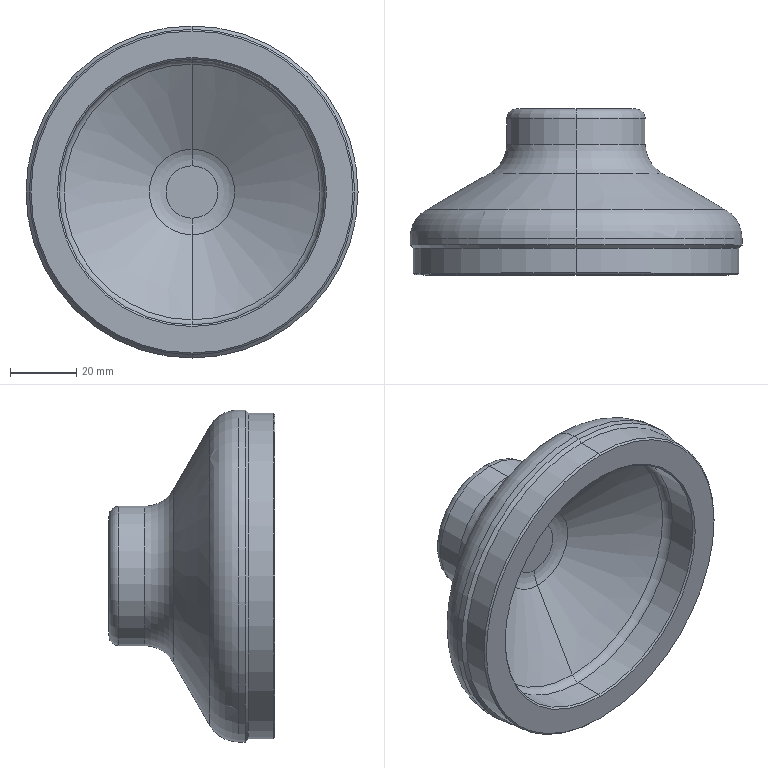Part | NX | features BREP 1 | 1 solid | 38 faces | box 100 x 50 x 100 mm | volume 123774 mm3 | cone 12 | cylinder 10 | torus 10 | plane 4 | sphere 2 | commonest cylinder face diameters 28 x2 42 x2 80 x2 98 x2 100 x2
STEP:
#1=CARTESIAN_POINT('',(0.,-49.5,40.));
#2=VERTEX_POINT('',#1);
#3=CARTESIAN_POINT('',(0.,-49.5,-40.));
#4=VERTEX_POINT('',#3);
#5=CARTESIAN_POINT('',(0.,-49.5,0.));
#6=DIRECTION('',(0.,-1.,0.));
#7=DIRECTION('',(0.,0.,1.));
#8=AXIS2_PLACEMENT_3D('',#5,#6,#7);
#9=CIRCLE('',#8,40.);
#10=EDGE_CURVE('',#2,#4,#9,.T.);
#11=ORIENTED_EDGE('',*,*,#10,.F.);
#12=CARTESIAN_POINT('',(0.,-50.,40.5));
#13=VERTEX_POINT('',#12);
#14=CARTESIAN_POINT('',(0.,-50.,40.5));
#15=DIRECTION('',(0.,-0.7071,0.7071));
#16=VECTOR('',#15,1000.);
#17=LINE('',#14,#16);
#18=EDGE_CURVE('',#2,#13,#17,.T.);
#19=ORIENTED_EDGE('',*,*,#18,.T.);
#20=CARTESIAN_POINT('',(0.,-50.,-40.5));
#21=VERTEX_POINT('',#20);
#22=CARTESIAN_POINT('',(0.,-50.,0.));
#23=DIRECTION('',(0.,1.,0.));
#24=DIRECTION('',(0.,0.,1.));
#25=AXIS2_PLACEMENT_3D('',#22,#23,#24);
#26=CIRCLE('',#25,40.5);
#27=EDGE_CURVE('',#21,#13,#26,.T.);
#28=ORIENTED_EDGE('',*,*,#27,.F.);
#29=CARTESIAN_POINT('',(0.,-50.,-40.5));
#30=DIRECTION('',(0.,-0.7071,-0.7071));
#31=VECTOR('',#30,1000.);
#32=LINE('',#29,#31);
#33=EDGE_CURVE('',#4,#21,#32,.T.);
#34=ORIENTED_EDGE('',*,*,#33,.F.);
#35=EDGE_LOOP('',(#11,#19,#28,#34));
#36=FACE_BOUND('',#35,.T.);
#37=CARTESIAN_POINT('',(0.,-50.,0.));
#38=DIRECTION('',(0.,-1.,0.));
#39=DIRECTION('',(0.,0.,-1.));
#40=AXIS2_PLACEMENT_3D('',#37,#38,#39);
#41=CONICAL_SURFACE('',#40,40.5,0.7854);
#42=ADVANCED_FACE('',(#36),#41,.F.);
#43=CARTESIAN_POINT('',(0.,-50.,-48.5));
#44=VERTEX_POINT('',#43);
#45=CARTESIAN_POINT('',(0.,-50.,48.5));
#46=VERTEX_POINT('',#45);
#47=CARTESIAN_POINT('',(0.,-50.,0.));
#48=DIRECTION('',(0.,-1.,0.));
#49=DIRECTION('',(0.,0.,1.));
#50=AXIS2_PLACEMENT_3D('',#47,#48,#49);
#51=CIRCLE('',#50,48.5);
#52=EDGE_CURVE('',#44,#46,#51,.T.);
#53=ORIENTED_EDGE('',*,*,#52,.F.);
#54=CARTESIAN_POINT('',(0.,-49.5,-49.));
#55=VERTEX_POINT('',#54);
#56=CARTESIAN_POINT('',(0.,-50.,-48.5));
#57=DIRECTION('',(0.,0.7071,-0.7071));
#58=VECTOR('',#57,1000.);
#59=LINE('',#56,#58);
#60=EDGE_CURVE('',#55,#44,#59,.F.);
#61=ORIENTED_EDGE('',*,*,#60,.F.);
#62=CARTESIAN_POINT('',(0.,-49.5,49.));
#63=VERTEX_POINT('',#62);
#64=CARTESIAN_POINT('',(0.,-49.5,0.));
#65=DIRECTION('',(0.,1.,0.));
#66=DIRECTION('',(0.,0.,1.));
#67=AXIS2_PLACEMENT_3D('',#64,#65,#66);
#68=CIRCLE('',#67,49.);
#69=EDGE_CURVE('',#63,#55,#68,.T.);
#70=ORIENTED_EDGE('',*,*,#69,.F.);
#71=CARTESIAN_POINT('',(0.,-50.,48.5));
#72=DIRECTION('',(0.,0.7071,0.7071));
#73=VECTOR('',#72,1000.);
#74=LINE('',#71,#73);
#75=EDGE_CURVE('',#63,#46,#74,.F.);
#76=ORIENTED_EDGE('',*,*,#75,.T.);
#77=EDGE_LOOP('',(#53,#61,#70,#76));
#78=FACE_BOUND('',#77,.T.);
#79=CARTESIAN_POINT('',(0.,-50.,0.));
#80=DIRECTION('',(0.,1.,0.));
#81=DIRECTION('',(0.,0.,1.));
#82=AXIS2_PLACEMENT_3D('',#79,#80,#81);
#83=CONICAL_SURFACE('',#82,48.5,0.7854);
#84=ADVANCED_FACE('',(#78),#83,.T.);
#85=CARTESIAN_POINT('',(0.,-42.,-49.));
#86=VERTEX_POINT('',#85);
#87=CARTESIAN_POINT('',(0.,-42.,49.));
#88=VERTEX_POINT('',#87);
#89=CARTESIAN_POINT('',(0.,-42.,0.));
#90=DIRECTION('',(0.,-1.,0.));
#91=DIRECTION('',(0.,0.,-1.));
#92=AXIS2_PLACEMENT_3D('',#89,#90,#91);
#93=CIRCLE('',#92,49.);
#94=EDGE_CURVE('',#86,#88,#93,.T.);
#95=ORIENTED_EDGE('',*,*,#94,.F.);
#96=CARTESIAN_POINT('',(0.,-41.,-50.));
#97=VERTEX_POINT('',#96);
#98=CARTESIAN_POINT('',(0.,-42.,-49.));
#99=DIRECTION('',(0.,0.7071,-0.7071));
#100=VECTOR('',#99,1000.);
#101=LINE('',#98,#100);
#102=EDGE_CURVE('',#97,#86,#101,.F.);
#103=ORIENTED_EDGE('',*,*,#102,.F.);
#104=CARTESIAN_POINT('',(0.,-41.,50.));
#105=VERTEX_POINT('',#104);
#106=CARTESIAN_POINT('',(0.,-41.,0.));
#107=DIRECTION('',(0.,1.,0.));
#108=DIRECTION('',(0.,0.,-1.));
#109=AXIS2_PLACEMENT_3D('',#106,#107,#108);
#110=CIRCLE('',#109,50.);
#111=EDGE_CURVE('',#105,#97,#110,.T.);
#112=ORIENTED_EDGE('',*,*,#111,.F.);
#113=CARTESIAN_POINT('',(0.,-42.,49.));
#114=DIRECTION('',(0.,0.7071,0.7071));
#115=VECTOR('',#114,1000.);
#116=LINE('',#113,#115);
#117=EDGE_CURVE('',#105,#88,#116,.F.);
#118=ORIENTED_EDGE('',*,*,#117,.T.);
#119=EDGE_LOOP('',(#95,#103,#112,#118));
#120=FACE_BOUND('',#119,.T.);
#121=CARTESIAN_POINT('',(0.,-42.,0.));
#122=DIRECTION('',(0.,1.,0.));
#123=DIRECTION('',(0.,0.,1.));
#124=AXIS2_PLACEMENT_3D('',#121,#122,#123);
#125=CONICAL_SURFACE('',#124,49.,0.7854);
#126=ADVANCED_FACE('',(#120),#125,.T.);
#127=ORIENTED_EDGE('',*,*,#10,.T.);
#128=CARTESIAN_POINT('',(0.,-40.732,-40.));
#129=VERTEX_POINT('',#128);
#130=CARTESIAN_POINT('',(0.,0.,-40.));
#131=DIRECTION('',(0.,1.,0.));
#132=VECTOR('',#131,1000.);
#133=LINE('',#130,#132);
#134=EDGE_CURVE('',#129,#4,#133,.F.);
#135=ORIENTED_EDGE('',*,*,#134,.F.);
#136=CARTESIAN_POINT('',(0.,-40.732,40.));
#137=VERTEX_POINT('',#136);
#138=CARTESIAN_POINT('',(0.,-40.732,0.));
#139=DIRECTION('',(0.,1.,0.));
#140=DIRECTION('',(0.,0.,1.));
#141=AXIS2_PLACEMENT_3D('',#138,#139,#140);
#142=CIRCLE('',#141,40.);
#143=EDGE_CURVE('',#129,#137,#142,.T.);
#144=ORIENTED_EDGE('',*,*,#143,.T.);
#145=CARTESIAN_POINT('',(0.,0.,40.));
#146=DIRECTION('',(0.,1.,0.));
#147=VECTOR('',#146,1000.);
#148=LINE('',#145,#147);
#149=EDGE_CURVE('',#137,#2,#148,.F.);
#150=ORIENTED_EDGE('',*,*,#149,.T.);
#151=EDGE_LOOP('',(#127,#135,#144,#150));
#152=FACE_BOUND('',#151,.T.);
#153=CARTESIAN_POINT('',(0.,0.,0.));
#154=DIRECTION('',(0.,1.,0.));
#155=DIRECTION('',(0.,0.,1.));
#156=AXIS2_PLACEMENT_3D('',#153,#154,#155);
#157=CYLINDRICAL_SURFACE('',#156,40.);
#158=ADVANCED_FACE('',(#152),#157,.F.);
#159=ORIENTED_EDGE('',*,*,#143,.F.);
#160=CARTESIAN_POINT('',(0.,-38.134,-38.5));
#161=VERTEX_POINT('',#160);
#162=CARTESIAN_POINT('',(0.,-40.732,-37.));
#163=DIRECTION('',(1.,0.,0.));
#164=DIRECTION('',(0.,0.,-1.));
#165=AXIS2_PLACEMENT_3D('',#162,#163,#164);
#166=CIRCLE('',#165,3.);
#167=EDGE_CURVE('',#161,#129,#166,.F.);
#168=ORIENTED_EDGE('',*,*,#167,.F.);
#169=CARTESIAN_POINT('',(0.,-38.134,38.5));
#170=VERTEX_POINT('',#169);
#171=CARTESIAN_POINT('',(0.,-38.134,0.));
#172=DIRECTION('',(0.,-1.,0.));
#173=DIRECTION('',(0.,0.,-1.));
#174=AXIS2_PLACEMENT_3D('',#171,#172,#173);
#175=CIRCLE('',#174,38.5);
#176=EDGE_CURVE('',#170,#161,#175,.T.);
#177=ORIENTED_EDGE('',*,*,#176,.F.);
#178=CARTESIAN_POINT('',(0.,-40.732,37.));
#179=DIRECTION('',(-1.,0.,0.));
#180=DIRECTION('',(0.,0.,1.));
#181=AXIS2_PLACEMENT_3D('',#178,#179,#180);
#182=CIRCLE('',#181,3.);
#183=EDGE_CURVE('',#170,#137,#182,.F.);
#184=ORIENTED_EDGE('',*,*,#183,.T.);
#185=EDGE_LOOP('',(#159,#168,#177,#184));
#186=FACE_BOUND('',#185,.T.);
#187=CARTESIAN_POINT('',(0.,-40.732,0.));
#188=DIRECTION('',(0.,1.,0.));
#189=DIRECTION('',(0.,0.,1.));
#190=AXIS2_PLACEMENT_3D('',#187,#188,#189);
#191=TOROIDAL_SURFACE('',#190,37.,3.);
#192=ADVANCED_FACE('',(#186),#191,.F.);
#193=CARTESIAN_POINT('',(0.,-23.34,-12.876));
#194=VERTEX_POINT('',#193);
#195=CARTESIAN_POINT('',(0.,-23.34,12.876));
#196=VERTEX_POINT('',#195);
#197=CARTESIAN_POINT('',(0.,-23.34,0.));
#198=DIRECTION('',(0.,1.,0.));
#199=DIRECTION('',(0.,0.,-1.));
#200=AXIS2_PLACEMENT_3D('',#197,#198,#199);
#201=CIRCLE('',#200,12.876);
#202=EDGE_CURVE('',#194,#196,#201,.T.);
#203=ORIENTED_EDGE('',*,*,#202,.T.);
#204=CARTESIAN_POINT('',(0.,-22.,10.555));
#205=DIRECTION('',(0.,-0.5,0.866));
#206=VECTOR('',#205,1000.);
#207=LINE('',#204,#206);
#208=EDGE_CURVE('',#196,#170,#207,.T.);
#209=ORIENTED_EDGE('',*,*,#208,.T.);
#210=ORIENTED_EDGE('',*,*,#176,.T.);
#211=CARTESIAN_POINT('',(0.,-22.,-10.555));
#212=DIRECTION('',(0.,-0.5,-0.866));
#213=VECTOR('',#212,1000.);
#214=LINE('',#211,#213);
#215=EDGE_CURVE('',#194,#161,#214,.T.);
#216=ORIENTED_EDGE('',*,*,#215,.F.);
#217=EDGE_LOOP('',(#203,#209,#210,#216));
#218=FACE_BOUND('',#217,.T.);
#219=CARTESIAN_POINT('',(0.,-22.,0.));
#220=DIRECTION('',(0.,-1.,0.));
#221=DIRECTION('',(0.,0.,-1.));
#222=AXIS2_PLACEMENT_3D('',#219,#220,#221);
#223=CONICAL_SURFACE('',#222,10.555,1.047);
#224=ADVANCED_FACE('',(#218),#223,.F.);
#225=ORIENTED_EDGE('',*,*,#202,.F.);
#226=CARTESIAN_POINT('',(0.,-22.,-7.876));
#227=VERTEX_POINT('',#226);
#228=CARTESIAN_POINT('',(0.,-32.,-7.876));
#229=DIRECTION('',(1.,0.,0.));
#230=DIRECTION('',(0.,0.,-1.));
#231=AXIS2_PLACEMENT_3D('',#228,#229,#230);
#232=CIRCLE('',#231,10.);
#233=EDGE_CURVE('',#227,#194,#232,.F.);
#234=ORIENTED_EDGE('',*,*,#233,.F.);
#235=CARTESIAN_POINT('',(0.,-22.,7.876));
#236=VERTEX_POINT('',#235);
#237=CARTESIAN_POINT('',(0.,-22.,0.));
#238=DIRECTION('',(0.,-1.,0.));
#239=DIRECTION('',(0.,0.,1.));
#240=AXIS2_PLACEMENT_3D('',#237,#238,#239);
#241=CIRCLE('',#240,7.876);
#242=EDGE_CURVE('',#236,#227,#241,.T.);
#243=ORIENTED_EDGE('',*,*,#242,.F.);
#244=CARTESIAN_POINT('',(0.,-32.,7.876));
#245=DIRECTION('',(-1.,0.,0.));
#246=DIRECTION('',(0.,0.,1.));
#247=AXIS2_PLACEMENT_3D('',#244,#245,#246);
#248=CIRCLE('',#247,10.);
#249=EDGE_CURVE('',#236,#196,#248,.F.);
#250=ORIENTED_EDGE('',*,*,#249,.T.);
#251=EDGE_LOOP('',(#225,#234,#243,#250));
#252=FACE_BOUND('',#251,.T.);
#253=CARTESIAN_POINT('',(0.,-32.,0.));
#254=DIRECTION('',(0.,1.,0.));
#255=DIRECTION('',(0.,0.,1.));
#256=AXIS2_PLACEMENT_3D('',#253,#254,#255);
#257=DEGENERATE_TOROIDAL_SURFACE('',#256,7.876,10.,.T.);
#258=ADVANCED_FACE('',(#252),#257,.F.);
#259=ORIENTED_EDGE('',*,*,#94,.T.);
#260=CARTESIAN_POINT('',(0.,-42.,49.));
#261=DIRECTION('',(0.,-1.,0.));
#262=VECTOR('',#261,1000.);
#263=LINE('',#260,#262);
#264=EDGE_CURVE('',#88,#63,#263,.T.);
#265=ORIENTED_EDGE('',*,*,#264,.T.);
#266=ORIENTED_EDGE('',*,*,#69,.T.);
#267=CARTESIAN_POINT('',(0.,-42.,-49.));
#268=DIRECTION('',(0.,-1.,0.));
#269=VECTOR('',#268,1000.);
#270=LINE('',#267,#269);
#271=EDGE_CURVE('',#86,#55,#270,.T.);
#272=ORIENTED_EDGE('',*,*,#271,.F.);
#273=EDGE_LOOP('',(#259,#265,#266,#272));
#274=FACE_BOUND('',#273,.T.);
#275=CARTESIAN_POINT('',(0.,-42.,0.));
#276=DIRECTION('',(0.,-1.,0.));
#277=DIRECTION('',(0.,0.,-1.));
#278=AXIS2_PLACEMENT_3D('',#275,#276,#277);
#279=CYLINDRICAL_SURFACE('',#278,49.);
#280=ADVANCED_FACE('',(#274),#279,.T.);
#281=CARTESIAN_POINT('',(0.,-1.508,-11.905));
#282=VERTEX_POINT('',#281);
#283=CARTESIAN_POINT('',(-11.905,-1.508,0.));
#284=VERTEX_POINT('',#283);
#285=CARTESIAN_POINT('',(0.,-1.508,0.));
#286=DIRECTION('',(0.,1.,0.));
#287=DIRECTION('',(0.,0.,1.));
#288=AXIS2_PLACEMENT_3D('',#285,#286,#287);
#289=CIRCLE('',#288,11.905);
#290=EDGE_CURVE('',#282,#284,#289,.T.);
#291=ORIENTED_EDGE('',*,*,#290,.F.);
#292=CARTESIAN_POINT('',(0.,-1.,-12.506));
#293=VERTEX_POINT('',#292);
#294=CARTESIAN_POINT('',(0.,-1.,-12.506));
#295=DIRECTION('',(0.,0.6457,-0.7636));
#296=VECTOR('',#295,1000.);
#297=LINE('',#294,#296);
#298=EDGE_CURVE('',#293,#282,#297,.F.);
#299=ORIENTED_EDGE('',*,*,#298,.F.);
#300=CARTESIAN_POINT('',(0.,-1.,12.506));
#301=VERTEX_POINT('',#300);
#302=CARTESIAN_POINT('',(0.,-1.,0.));
#303=DIRECTION('',(0.,-1.,0.));
#304=DIRECTION('',(0.,0.,1.));
#305=AXIS2_PLACEMENT_3D('',#302,#303,#304);
#306=CIRCLE('',#305,12.506);
#307=EDGE_CURVE('',#301,#293,#306,.T.);
#308=ORIENTED_EDGE('',*,*,#307,.F.);
#309=CARTESIAN_POINT('',(0.,-1.508,11.905));
#310=VERTEX_POINT('',#309);
#311=CARTESIAN_POINT('',(0.,-1.,12.506));
#312=DIRECTION('',(0.,0.6457,0.7636));
#313=VECTOR('',#312,1000.);
#314=LINE('',#311,#313);
#315=EDGE_CURVE('',#301,#310,#314,.F.);
#316=ORIENTED_EDGE('',*,*,#315,.T.);
#317=CARTESIAN_POINT('',(0.,-1.508,0.));
#318=DIRECTION('',(0.,1.,0.));
#319=DIRECTION('',(0.,0.,1.));
#320=AXIS2_PLACEMENT_3D('',#317,#318,#319);
#321=CIRCLE('',#320,11.905);
#322=EDGE_CURVE('',#284,#310,#321,.T.);
#323=ORIENTED_EDGE('',*,*,#322,.F.);
#324=EDGE_LOOP('',(#291,#299,#308,#316,#323));
#325=FACE_BOUND('',#324,.T.);
#326=CARTESIAN_POINT('',(0.,-1.,0.));
#327=DIRECTION('',(0.,1.,0.));
#328=DIRECTION('',(0.,0.,1.));
#329=AXIS2_PLACEMENT_3D('',#326,#327,#328);
#330=CONICAL_SURFACE('',#329,12.506,0.8688);
#331=ADVANCED_FACE('',(#325),#330,.F.);
#332=CARTESIAN_POINT('',(11.905,-1.508,0.));
#333=VERTEX_POINT('',#332);
#334=CARTESIAN_POINT('',(0.,0.,0.));
#335=DIRECTION('',(0.,0.,1.));
#336=DIRECTION('',(1.,0.,0.));
#337=AXIS2_PLACEMENT_3D('',#334,#335,#336);
#338=CIRCLE('',#337,12.);
#339=EDGE_CURVE('',#284,#333,#338,.T.);
#340=ORIENTED_EDGE('',*,*,#339,.F.);
#341=ORIENTED_EDGE('',*,*,#322,.T.);
#342=CARTESIAN_POINT('',(0.,-1.508,0.));
#343=DIRECTION('',(0.,1.,0.));
#344=DIRECTION('',(0.,0.,1.));
#345=AXIS2_PLACEMENT_3D('',#342,#343,#344);
#346=CIRCLE('',#345,11.905);
#347=EDGE_CURVE('',#310,#333,#346,.T.);
#348=ORIENTED_EDGE('',*,*,#347,.T.);
#349=EDGE_LOOP('',(#340,#341,#348));
#350=FACE_BOUND('',#349,.T.);
#351=CARTESIAN_POINT('',(0.,0.,0.));
#352=DIRECTION('',(0.,-1.,0.));
#353=DIRECTION('',(1.,0.,0.));
#354=AXIS2_PLACEMENT_3D('',#351,#352,#353);
#355=SPHERICAL_SURFACE('',#354,12.);
#356=ADVANCED_FACE('',(#350),#355,.F.);
#357=CARTESIAN_POINT('',(0.,-1.,-14.));
#358=VERTEX_POINT('',#357);
#359=CARTESIAN_POINT('',(0.,-1.,14.));
#360=VERTEX_POINT('',#359);
#361=CARTESIAN_POINT('',(0.,-1.,0.));
#362=DIRECTION('',(0.,1.,0.));
#363=DIRECTION('',(0.,0.,1.));
#364=AXIS2_PLACEMENT_3D('',#361,#362,#363);
#365=CIRCLE('',#364,14.);
#366=EDGE_CURVE('',#358,#360,#365,.T.);
#367=ORIENTED_EDGE('',*,*,#366,.F.);
#368=CARTESIAN_POINT('',(0.,0.,-14.));
#369=VERTEX_POINT('',#368);
#370=CARTESIAN_POINT('',(0.,-1.,-14.));
#371=DIRECTION('',(0.,1.,0.));
#372=VECTOR('',#371,1000.);
#373=LINE('',#370,#372);
#374=EDGE_CURVE('',#369,#358,#373,.F.);
#375=ORIENTED_EDGE('',*,*,#374,.F.);
#376=CARTESIAN_POINT('',(0.,0.,14.));
#377=VERTEX_POINT('',#376);
#378=CARTESIAN_POINT('',(0.,0.,0.));
#379=DIRECTION('',(0.,1.,0.));
#380=DIRECTION('',(0.,0.,1.));
#381=AXIS2_PLACEMENT_3D('',#378,#379,#380);
#382=CIRCLE('',#381,14.);
#383=EDGE_CURVE('',#369,#377,#382,.T.);
#384=ORIENTED_EDGE('',*,*,#383,.T.);
#385=CARTESIAN_POINT('',(0.,-1.,14.));
#386=DIRECTION('',(0.,1.,0.));
#387=VECTOR('',#386,1000.);
#388=LINE('',#385,#387);
#389=EDGE_CURVE('',#377,#360,#388,.F.);
#390=ORIENTED_EDGE('',*,*,#389,.T.);
#391=EDGE_LOOP('',(#367,#375,#384,#390));
#392=FACE_BOUND('',#391,.T.);
#393=CARTESIAN_POINT('',(0.,-1.,0.));
#394=DIRECTION('',(0.,1.,0.));
#395=DIRECTION('',(0.,0.,1.));
#396=AXIS2_PLACEMENT_3D('',#393,#394,#395);
#397=CYLINDRICAL_SURFACE('',#396,14.);
#398=ADVANCED_FACE('',(#392),#397,.F.);
#399=CARTESIAN_POINT('',(0.,-10.71,-21.));
#400=VERTEX_POINT('',#399);
#401=CARTESIAN_POINT('',(0.,-10.71,21.));
#402=VERTEX_POINT('',#401);
#403=CARTESIAN_POINT('',(0.,-10.71,0.));
#404=DIRECTION('',(0.,1.,0.));
#405=DIRECTION('',(0.,0.,1.));
#406=AXIS2_PLACEMENT_3D('',#403,#404,#405);
#407=CIRCLE('',#406,21.);
#408=EDGE_CURVE('',#400,#402,#407,.T.);
#409=ORIENTED_EDGE('',*,*,#408,.F.);
#410=CARTESIAN_POINT('',(0.,-19.37,-26.));
#411=VERTEX_POINT('',#410);
#412=CARTESIAN_POINT('',(0.,-10.71,-31.));
#413=DIRECTION('',(1.,0.,0.));
#414=DIRECTION('',(0.,0.,-1.));
#415=AXIS2_PLACEMENT_3D('',#412,#413,#414);
#416=CIRCLE('',#415,10.);
#417=EDGE_CURVE('',#411,#400,#416,.F.);
#418=ORIENTED_EDGE('',*,*,#417,.F.);
#419=CARTESIAN_POINT('',(0.,-19.37,26.));
#420=VERTEX_POINT('',#419);
#421=CARTESIAN_POINT('',(0.,-19.37,0.));
#422=DIRECTION('',(0.,-1.,0.));
#423=DIRECTION('',(0.,0.,-1.));
#424=AXIS2_PLACEMENT_3D('',#421,#422,#423);
#425=CIRCLE('',#424,26.);
#426=EDGE_CURVE('',#420,#411,#425,.T.);
#427=ORIENTED_EDGE('',*,*,#426,.F.);
#428=CARTESIAN_POINT('',(0.,-10.71,31.));
#429=DIRECTION('',(-1.,0.,0.));
#430=DIRECTION('',(0.,0.,1.));
#431=AXIS2_PLACEMENT_3D('',#428,#429,#430);
#432=CIRCLE('',#431,10.);
#433=EDGE_CURVE('',#420,#402,#432,.F.);
#434=ORIENTED_EDGE('',*,*,#433,.T.);
#435=EDGE_LOOP('',(#409,#418,#427,#434));
#436=FACE_BOUND('',#435,.T.);
#437=CARTESIAN_POINT('',(0.,-10.71,0.));
#438=DIRECTION('',(0.,1.,0.));
#439=DIRECTION('',(0.,0.,1.));
#440=AXIS2_PLACEMENT_3D('',#437,#438,#439);
#441=TOROIDAL_SURFACE('',#440,31.,10.);
#442=ADVANCED_FACE('',(#436),#441,.F.);
#443=CARTESIAN_POINT('',(0.,-30.34,45.));
#444=VERTEX_POINT('',#443);
#445=CARTESIAN_POINT('',(0.,-30.34,-45.));
#446=VERTEX_POINT('',#445);
#447=CARTESIAN_POINT('',(0.,-30.34,0.));
#448=DIRECTION('',(0.,1.,0.));
#449=DIRECTION('',(0.,0.,1.));
#450=AXIS2_PLACEMENT_3D('',#447,#448,#449);
#451=CIRCLE('',#450,45.);
#452=EDGE_CURVE('',#444,#446,#451,.T.);
#453=ORIENTED_EDGE('',*,*,#452,.F.);
#454=CARTESIAN_POINT('',(0.,-39.,50.));
#455=VERTEX_POINT('',#454);
#456=CARTESIAN_POINT('',(0.,-39.,40.));
#457=DIRECTION('',(1.,0.,0.));
#458=DIRECTION('',(0.,0.,-1.));
#459=AXIS2_PLACEMENT_3D('',#456,#457,#458);
#460=CIRCLE('',#459,10.);
#461=EDGE_CURVE('',#444,#455,#460,.T.);
#462=ORIENTED_EDGE('',*,*,#461,.T.);
#463=CARTESIAN_POINT('',(0.,-39.,-50.));
#464=VERTEX_POINT('',#463);
#465=CARTESIAN_POINT('',(0.,-39.,0.));
#466=DIRECTION('',(0.,-1.,0.));
#467=DIRECTION('',(0.,0.,-1.));
#468=AXIS2_PLACEMENT_3D('',#465,#466,#467);
#469=CIRCLE('',#468,50.);
#470=EDGE_CURVE('',#464,#455,#469,.T.);
#471=ORIENTED_EDGE('',*,*,#470,.F.);
#472=CARTESIAN_POINT('',(0.,-39.,-40.));
#473=DIRECTION('',(-1.,0.,0.));
#474=DIRECTION('',(0.,0.,1.));
#475=AXIS2_PLACEMENT_3D('',#472,#473,#474);
#476=CIRCLE('',#475,10.);
#477=EDGE_CURVE('',#446,#464,#476,.T.);
#478=ORIENTED_EDGE('',*,*,#477,.F.);
#479=EDGE_LOOP('',(#453,#462,#471,#478));
#480=FACE_BOUND('',#479,.T.);
#481=CARTESIAN_POINT('',(0.,-39.,0.));
#482=DIRECTION('',(0.,-1.,0.));
#483=DIRECTION('',(0.,0.,-1.));
#484=AXIS2_PLACEMENT_3D('',#481,#482,#483);
#485=TOROIDAL_SURFACE('',#484,40.,10.);
#486=ADVANCED_FACE('',(#480),#485,.T.);
#487=CARTESIAN_POINT('',(0.,0.,18.));
#488=VERTEX_POINT('',#487);
#489=CARTESIAN_POINT('',(0.,0.,-18.));
#490=VERTEX_POINT('',#489);
#491=CARTESIAN_POINT('',(0.,0.,0.));
#492=DIRECTION('',(0.,1.,0.));
#493=DIRECTION('',(0.,0.,-1.));
#494=AXIS2_PLACEMENT_3D('',#491,#492,#493);
#495=CIRCLE('',#494,18.);
#496=EDGE_CURVE('',#488,#490,#495,.T.);
#497=ORIENTED_EDGE('',*,*,#496,.F.);
#498=CARTESIAN_POINT('',(0.,-3.,21.));
#499=VERTEX_POINT('',#498);
#500=CARTESIAN_POINT('',(0.,-3.,18.));
#501=DIRECTION('',(1.,0.,0.));
#502=DIRECTION('',(0.,0.,-1.));
#503=AXIS2_PLACEMENT_3D('',#500,#501,#502);
#504=CIRCLE('',#503,3.);
#505=EDGE_CURVE('',#488,#499,#504,.T.);
#506=ORIENTED_EDGE('',*,*,#505,.T.);
#507=CARTESIAN_POINT('',(0.,-3.,-21.));
#508=VERTEX_POINT('',#507);
#509=CARTESIAN_POINT('',(0.,-3.,0.));
#510=DIRECTION('',(0.,-1.,0.));
#511=DIRECTION('',(0.,0.,-1.));
#512=AXIS2_PLACEMENT_3D('',#509,#510,#511);
#513=CIRCLE('',#512,21.);
#514=EDGE_CURVE('',#508,#499,#513,.T.);
#515=ORIENTED_EDGE('',*,*,#514,.F.);
#516=CARTESIAN_POINT('',(0.,-3.,-18.));
#517=DIRECTION('',(-1.,0.,0.));
#518=DIRECTION('',(0.,0.,1.));
#519=AXIS2_PLACEMENT_3D('',#516,#517,#518);
#520=CIRCLE('',#519,3.);
#521=EDGE_CURVE('',#490,#508,#520,.T.);
#522=ORIENTED_EDGE('',*,*,#521,.F.);
#523=EDGE_LOOP('',(#497,#506,#515,#522));
#524=FACE_BOUND('',#523,.T.);
#525=CARTESIAN_POINT('',(0.,-3.,0.));
#526=DIRECTION('',(0.,-1.,0.));
#527=DIRECTION('',(0.,0.,-1.));
#528=AXIS2_PLACEMENT_3D('',#525,#526,#527);
#529=TOROIDAL_SURFACE('',#528,18.,3.);
#530=ADVANCED_FACE('',(#524),#529,.T.);
#531=CARTESIAN_POINT('',(0.,-10.71,0.));
#532=DIRECTION('',(0.,1.,0.));
#533=DIRECTION('',(0.,0.,1.));
#534=AXIS2_PLACEMENT_3D('',#531,#532,#533);
#535=CIRCLE('',#534,21.);
#536=EDGE_CURVE('',#402,#400,#535,.T.);
#537=ORIENTED_EDGE('',*,*,#536,.T.);
#538=CARTESIAN_POINT('',(0.,0.,-21.));
#539=DIRECTION('',(0.,1.,0.));
#540=VECTOR('',#539,1000.);
#541=LINE('',#538,#540);
#542=EDGE_CURVE('',#508,#400,#541,.F.);
#543=ORIENTED_EDGE('',*,*,#542,.F.);
#544=ORIENTED_EDGE('',*,*,#514,.T.);
#545=CARTESIAN_POINT('',(0.,0.,21.));
#546=DIRECTION('',(0.,1.,0.));
#547=VECTOR('',#546,1000.);
#548=LINE('',#545,#547);
#549=EDGE_CURVE('',#499,#402,#548,.F.);
#550=ORIENTED_EDGE('',*,*,#549,.T.);
#551=EDGE_LOOP('',(#537,#543,#544,#550));
#552=FACE_BOUND('',#551,.T.);
#553=CARTESIAN_POINT('',(0.,0.,0.));
#554=DIRECTION('',(0.,1.,0.));
#555=DIRECTION('',(0.,0.,1.));
#556=AXIS2_PLACEMENT_3D('',#553,#554,#555);
#557=CYLINDRICAL_SURFACE('',#556,21.);
#558=ADVANCED_FACE('',(#552),#557,.T.);
#559=CARTESIAN_POINT('',(0.,-19.37,0.));
#560=DIRECTION('',(0.,-1.,0.));
#561=DIRECTION('',(0.,0.,-1.));
#562=AXIS2_PLACEMENT_3D('',#559,#560,#561);
#563=CIRCLE('',#562,26.);
#564=EDGE_CURVE('',#411,#420,#563,.T.);
#565=ORIENTED_EDGE('',*,*,#564,.T.);
#566=CARTESIAN_POINT('',(0.,-33.226,50.));
#567=DIRECTION('',(0.,-0.5,0.866));
#568=VECTOR('',#567,1000.);
#569=LINE('',#566,#568);
#570=EDGE_CURVE('',#420,#444,#569,.T.);
#571=ORIENTED_EDGE('',*,*,#570,.T.);
#572=ORIENTED_EDGE('',*,*,#452,.T.);
#573=CARTESIAN_POINT('',(0.,-33.226,-50.));
#574=DIRECTION('',(0.,-0.5,-0.866));
#575=VECTOR('',#574,1000.);
#576=LINE('',#573,#575);
#577=EDGE_CURVE('',#411,#446,#576,.T.);
#578=ORIENTED_EDGE('',*,*,#577,.F.);
#579=EDGE_LOOP('',(#565,#571,#572,#578));
#580=FACE_BOUND('',#579,.T.);
#581=CARTESIAN_POINT('',(0.,-33.226,0.));
#582=DIRECTION('',(0.,-1.,0.));
#583=DIRECTION('',(0.,0.,-1.));
#584=AXIS2_PLACEMENT_3D('',#581,#582,#583);
#585=CONICAL_SURFACE('',#584,50.,1.047);
#586=ADVANCED_FACE('',(#580),#585,.T.);
#587=ORIENTED_EDGE('',*,*,#111,.T.);
#588=CARTESIAN_POINT('',(0.,0.,-50.));
#589=DIRECTION('',(0.,1.,0.));
#590=VECTOR('',#589,1000.);
#591=LINE('',#588,#590);
#592=EDGE_CURVE('',#464,#97,#591,.F.);
#593=ORIENTED_EDGE('',*,*,#592,.F.);
#594=ORIENTED_EDGE('',*,*,#470,.T.);
#595=CARTESIAN_POINT('',(0.,0.,50.));
#596=DIRECTION('',(0.,1.,0.));
#597=VECTOR('',#596,1000.);
#598=LINE('',#595,#597);
#599=EDGE_CURVE('',#455,#105,#598,.F.);
#600=ORIENTED_EDGE('',*,*,#599,.T.);
#601=EDGE_LOOP('',(#587,#593,#594,#600));
#602=FACE_BOUND('',#601,.T.);
#603=CARTESIAN_POINT('',(0.,0.,0.));
#604=DIRECTION('',(0.,1.,0.));
#605=DIRECTION('',(0.,0.,1.));
#606=AXIS2_PLACEMENT_3D('',#603,#604,#605);
#607=CYLINDRICAL_SURFACE('',#606,50.);
#608=ADVANCED_FACE('',(#602),#607,.T.);
#609=ORIENTED_EDGE('',*,*,#592,.T.);
#610=CARTESIAN_POINT('',(0.,-41.,0.));
#611=DIRECTION('',(0.,1.,0.));
#612=DIRECTION('',(0.,0.,-1.));
#613=AXIS2_PLACEMENT_3D('',#610,#611,#612);
#614=CIRCLE('',#613,50.);
#615=EDGE_CURVE('',#97,#105,#614,.T.);
#616=ORIENTED_EDGE('',*,*,#615,.T.);
#617=ORIENTED_EDGE('',*,*,#599,.F.);
#618=CARTESIAN_POINT('',(0.,-39.,0.));
#619=DIRECTION('',(0.,-1.,0.));
#620=DIRECTION('',(0.,0.,-1.));
#621=AXIS2_PLACEMENT_3D('',#618,#619,#620);
#622=CIRCLE('',#621,50.);
#623=EDGE_CURVE('',#455,#464,#622,.T.);
#624=ORIENTED_EDGE('',*,*,#623,.T.);
#625=EDGE_LOOP('',(#609,#616,#617,#624));
#626=FACE_BOUND('',#625,.T.);
#627=CARTESIAN_POINT('',(0.,0.,0.));
#628=DIRECTION('',(0.,1.,0.));
#629=DIRECTION('',(0.,0.,1.));
#630=AXIS2_PLACEMENT_3D('',#627,#628,#629);
#631=CYLINDRICAL_SURFACE('',#630,50.);
#632=ADVANCED_FACE('',(#626),#631,.T.);
#633=ORIENTED_EDGE('',*,*,#570,.F.);
#634=ORIENTED_EDGE('',*,*,#426,.T.);
#635=ORIENTED_EDGE('',*,*,#577,.T.);
#636=CARTESIAN_POINT('',(0.,-30.34,0.));
#637=DIRECTION('',(0.,1.,0.));
#638=DIRECTION('',(0.,0.,1.));
#639=AXIS2_PLACEMENT_3D('',#636,#637,#638);
#640=CIRCLE('',#639,45.);
#641=EDGE_CURVE('',#446,#444,#640,.T.);
#642=ORIENTED_EDGE('',*,*,#641,.T.);
#643=EDGE_LOOP('',(#633,#634,#635,#642));
#644=FACE_BOUND('',#643,.T.);
#645=CARTESIAN_POINT('',(0.,-33.226,0.));
#646=DIRECTION('',(0.,-1.,0.));
#647=DIRECTION('',(0.,0.,-1.));
#648=AXIS2_PLACEMENT_3D('',#645,#646,#647);
#649=CONICAL_SURFACE('',#648,50.,1.047);
#650=ADVANCED_FACE('',(#644),#649,.T.);
#651=ORIENTED_EDGE('',*,*,#542,.T.);
#652=ORIENTED_EDGE('',*,*,#408,.T.);
#653=ORIENTED_EDGE('',*,*,#549,.F.);
#654=CARTESIAN_POINT('',(0.,-3.,0.));
#655=DIRECTION('',(0.,-1.,0.));
#656=DIRECTION('',(0.,0.,-1.));
#657=AXIS2_PLACEMENT_3D('',#654,#655,#656);
#658=CIRCLE('',#657,21.);
#659=EDGE_CURVE('',#499,#508,#658,.T.);
#660=ORIENTED_EDGE('',*,*,#659,.T.);
#661=EDGE_LOOP('',(#651,#652,#653,#660));
#662=FACE_BOUND('',#661,.T.);
#663=CARTESIAN_POINT('',(0.,0.,0.));
#664=DIRECTION('',(0.,1.,0.));
#665=DIRECTION('',(0.,0.,1.));
#666=AXIS2_PLACEMENT_3D('',#663,#664,#665);
#667=CYLINDRICAL_SURFACE('',#666,21.);
#668=ADVANCED_FACE('',(#662),#667,.T.);
#669=CARTESIAN_POINT('',(0.,0.,0.));
#670=DIRECTION('',(0.,1.,0.));
#671=DIRECTION('',(0.,0.,-1.));
#672=AXIS2_PLACEMENT_3D('',#669,#670,#671);
#673=CIRCLE('',#672,18.);
#674=EDGE_CURVE('',#490,#488,#673,.T.);
#675=ORIENTED_EDGE('',*,*,#674,.T.);
#676=ORIENTED_EDGE('',*,*,#496,.T.);
#677=EDGE_LOOP('',(#675,#676));
#678=FACE_BOUND('',#677,.T.);
#679=CARTESIAN_POINT('',(0.,0.,0.));
#680=DIRECTION('',(0.,1.,0.));
#681=DIRECTION('',(0.,0.,1.));
#682=AXIS2_PLACEMENT_3D('',#679,#680,#681);
#683=CIRCLE('',#682,14.);
#684=EDGE_CURVE('',#377,#369,#683,.T.);
#685=ORIENTED_EDGE('',*,*,#684,.F.);
#686=ORIENTED_EDGE('',*,*,#383,.F.);
#687=EDGE_LOOP('',(#685,#686));
#688=FACE_BOUND('',#687,.T.);
#689=CARTESIAN_POINT('',(21.,0.,0.));
#690=DIRECTION('',(0.,-1.,0.));
#691=DIRECTION('',(0.,0.,-1.));
#692=AXIS2_PLACEMENT_3D('',#689,#690,#691);
#693=PLANE('',#692);
#694=ADVANCED_FACE('',(#678,#688),#693,.F.);
#695=ORIENTED_EDGE('',*,*,#505,.F.);
#696=ORIENTED_EDGE('',*,*,#674,.F.);
#697=ORIENTED_EDGE('',*,*,#521,.T.);
#698=ORIENTED_EDGE('',*,*,#659,.F.);
#699=EDGE_LOOP('',(#695,#696,#697,#698));
#700=FACE_BOUND('',#699,.T.);
#701=CARTESIAN_POINT('',(0.,-3.,0.));
#702=DIRECTION('',(0.,-1.,0.));
#703=DIRECTION('',(0.,0.,-1.));
#704=AXIS2_PLACEMENT_3D('',#701,#702,#703);
#705=TOROIDAL_SURFACE('',#704,18.,3.);
#706=ADVANCED_FACE('',(#700),#705,.T.);
#707=ORIENTED_EDGE('',*,*,#461,.F.);
#708=ORIENTED_EDGE('',*,*,#641,.F.);
#709=ORIENTED_EDGE('',*,*,#477,.T.);
#710=ORIENTED_EDGE('',*,*,#623,.F.);
#711=EDGE_LOOP('',(#707,#708,#709,#710));
#712=FACE_BOUND('',#711,.T.);
#713=CARTESIAN_POINT('',(0.,-39.,0.));
#714=DIRECTION('',(0.,-1.,0.));
#715=DIRECTION('',(0.,0.,-1.));
#716=AXIS2_PLACEMENT_3D('',#713,#714,#715);
#717=TOROIDAL_SURFACE('',#716,40.,10.);
#718=ADVANCED_FACE('',(#712),#717,.T.);
#719=ORIENTED_EDGE('',*,*,#417,.T.);
#720=ORIENTED_EDGE('',*,*,#536,.F.);
#721=ORIENTED_EDGE('',*,*,#433,.F.);
#722=ORIENTED_EDGE('',*,*,#564,.F.);
#723=EDGE_LOOP('',(#719,#720,#721,#722));
#724=FACE_BOUND('',#723,.T.);
#725=CARTESIAN_POINT('',(0.,-10.71,0.));
#726=DIRECTION('',(0.,1.,0.));
#727=DIRECTION('',(0.,0.,1.));
#728=AXIS2_PLACEMENT_3D('',#725,#726,#727);
#729=TOROIDAL_SURFACE('',#728,31.,10.);
#730=ADVANCED_FACE('',(#724),#729,.F.);
#731=CARTESIAN_POINT('',(0.,-1.,0.));
#732=DIRECTION('',(0.,1.,0.));
#733=DIRECTION('',(0.,0.,1.));
#734=AXIS2_PLACEMENT_3D('',#731,#732,#733);
#735=CIRCLE('',#734,14.);
#736=EDGE_CURVE('',#360,#358,#735,.T.);
#737=ORIENTED_EDGE('',*,*,#736,.T.);
#738=ORIENTED_EDGE('',*,*,#366,.T.);
#739=EDGE_LOOP('',(#737,#738));
#740=FACE_BOUND('',#739,.T.);
#741=ORIENTED_EDGE('',*,*,#307,.T.);
#742=CARTESIAN_POINT('',(0.,-1.,0.));
#743=DIRECTION('',(0.,-1.,0.));
#744=DIRECTION('',(0.,0.,1.));
#745=AXIS2_PLACEMENT_3D('',#742,#743,#744);
#746=CIRCLE('',#745,12.506);
#747=EDGE_CURVE('',#293,#301,#746,.T.);
#748=ORIENTED_EDGE('',*,*,#747,.T.);
#749=EDGE_LOOP('',(#741,#748));
#750=FACE_BOUND('',#749,.T.);
#751=CARTESIAN_POINT('',(0.,-1.,0.));
#752=DIRECTION('',(0.,1.,0.));
#753=DIRECTION('',(1.,0.,0.));
#754=AXIS2_PLACEMENT_3D('',#751,#752,#753);
#755=PLANE('',#754);
#756=ADVANCED_FACE('',(#740,#750),#755,.T.);
#757=ORIENTED_EDGE('',*,*,#374,.T.);
#758=ORIENTED_EDGE('',*,*,#736,.F.);
#759=ORIENTED_EDGE('',*,*,#389,.F.);
#760=ORIENTED_EDGE('',*,*,#684,.T.);
#761=EDGE_LOOP('',(#757,#758,#759,#760));
#762=FACE_BOUND('',#761,.T.);
#763=CARTESIAN_POINT('',(0.,-1.,0.));
#764=DIRECTION('',(0.,1.,0.));
#765=DIRECTION('',(0.,0.,1.));
#766=AXIS2_PLACEMENT_3D('',#763,#764,#765);
#767=CYLINDRICAL_SURFACE('',#766,14.);
#768=ADVANCED_FACE('',(#762),#767,.F.);
#769=ORIENTED_EDGE('',*,*,#290,.T.);
#770=ORIENTED_EDGE('',*,*,#339,.T.);
#771=CARTESIAN_POINT('',(0.,-1.508,0.));
#772=DIRECTION('',(0.,1.,0.));
#773=DIRECTION('',(0.,0.,1.));
#774=AXIS2_PLACEMENT_3D('',#771,#772,#773);
#775=CIRCLE('',#774,11.905);
#776=EDGE_CURVE('',#333,#282,#775,.T.);
#777=ORIENTED_EDGE('',*,*,#776,.T.);
#778=EDGE_LOOP('',(#769,#770,#777));
#779=FACE_BOUND('',#778,.T.);
#780=CARTESIAN_POINT('',(0.,0.,0.));
#781=DIRECTION('',(0.,-1.,0.));
#782=DIRECTION('',(1.,0.,0.));
#783=AXIS2_PLACEMENT_3D('',#780,#781,#782);
#784=SPHERICAL_SURFACE('',#783,12.);
#785=ADVANCED_FACE('',(#779),#784,.F.);
#786=ORIENTED_EDGE('',*,*,#298,.T.);
#787=ORIENTED_EDGE('',*,*,#776,.F.);
#788=ORIENTED_EDGE('',*,*,#347,.F.);
#789=ORIENTED_EDGE('',*,*,#315,.F.);
#790=ORIENTED_EDGE('',*,*,#747,.F.);
#791=EDGE_LOOP('',(#786,#787,#788,#789,#790));
#792=FACE_BOUND('',#791,.T.);
#793=CARTESIAN_POINT('',(0.,-1.,0.));
#794=DIRECTION('',(0.,1.,0.));
#795=DIRECTION('',(0.,0.,1.));
#796=AXIS2_PLACEMENT_3D('',#793,#794,#795);
#797=CONICAL_SURFACE('',#796,12.506,0.8688);
#798=ADVANCED_FACE('',(#792),#797,.F.);
#799=ORIENTED_EDGE('',*,*,#264,.F.);
#800=CARTESIAN_POINT('',(0.,-42.,0.));
#801=DIRECTION('',(0.,-1.,0.));
#802=DIRECTION('',(0.,0.,-1.));
#803=AXIS2_PLACEMENT_3D('',#800,#801,#802);
#804=CIRCLE('',#803,49.);
#805=EDGE_CURVE('',#88,#86,#804,.T.);
#806=ORIENTED_EDGE('',*,*,#805,.T.);
#807=ORIENTED_EDGE('',*,*,#271,.T.);
#808=CARTESIAN_POINT('',(0.,-49.5,0.));
#809=DIRECTION('',(0.,1.,0.));
#810=DIRECTION('',(0.,0.,1.));
#811=AXIS2_PLACEMENT_3D('',#808,#809,#810);
#812=CIRCLE('',#811,49.);
#813=EDGE_CURVE('',#55,#63,#812,.T.);
#814=ORIENTED_EDGE('',*,*,#813,.T.);
#815=EDGE_LOOP('',(#799,#806,#807,#814));
#816=FACE_BOUND('',#815,.T.);
#817=CARTESIAN_POINT('',(0.,-42.,0.));
#818=DIRECTION('',(0.,-1.,0.));
#819=DIRECTION('',(0.,0.,-1.));
#820=AXIS2_PLACEMENT_3D('',#817,#818,#819);
#821=CYLINDRICAL_SURFACE('',#820,49.);
#822=ADVANCED_FACE('',(#816),#821,.T.);
#823=ORIENTED_EDGE('',*,*,#242,.T.);
#824=CARTESIAN_POINT('',(0.,-22.,0.));
#825=DIRECTION('',(0.,-1.,0.));
#826=DIRECTION('',(0.,0.,1.));
#827=AXIS2_PLACEMENT_3D('',#824,#825,#826);
#828=CIRCLE('',#827,7.876);
#829=EDGE_CURVE('',#227,#236,#828,.T.);
#830=ORIENTED_EDGE('',*,*,#829,.T.);
#831=EDGE_LOOP('',(#823,#830));
#832=FACE_BOUND('',#831,.T.);
#833=CARTESIAN_POINT('',(10.555,-22.,0.));
#834=DIRECTION('',(0.,1.,0.));
#835=DIRECTION('',(1.,0.,0.));
#836=AXIS2_PLACEMENT_3D('',#833,#834,#835);
#837=PLANE('',#836);
#838=ADVANCED_FACE('',(#832),#837,.F.);
#839=ORIENTED_EDGE('',*,*,#233,.T.);
#840=CARTESIAN_POINT('',(0.,-23.34,0.));
#841=DIRECTION('',(0.,1.,0.));
#842=DIRECTION('',(0.,0.,-1.));
#843=AXIS2_PLACEMENT_3D('',#840,#841,#842);
#844=CIRCLE('',#843,12.876);
#845=EDGE_CURVE('',#196,#194,#844,.T.);
#846=ORIENTED_EDGE('',*,*,#845,.F.);
#847=ORIENTED_EDGE('',*,*,#249,.F.);
#848=ORIENTED_EDGE('',*,*,#829,.F.);
#849=EDGE_LOOP('',(#839,#846,#847,#848));
#850=FACE_BOUND('',#849,.T.);
#851=CARTESIAN_POINT('',(0.,-32.,0.));
#852=DIRECTION('',(0.,1.,0.));
#853=DIRECTION('',(0.,0.,1.));
#854=AXIS2_PLACEMENT_3D('',#851,#852,#853);
#855=DEGENERATE_TOROIDAL_SURFACE('',#854,7.876,10.,.T.);
#856=ADVANCED_FACE('',(#850),#855,.F.);
#857=ORIENTED_EDGE('',*,*,#208,.F.);
#858=ORIENTED_EDGE('',*,*,#845,.T.);
#859=ORIENTED_EDGE('',*,*,#215,.T.);
#860=CARTESIAN_POINT('',(0.,-38.134,0.));
#861=DIRECTION('',(0.,-1.,0.));
#862=DIRECTION('',(0.,0.,-1.));
#863=AXIS2_PLACEMENT_3D('',#860,#861,#862);
#864=CIRCLE('',#863,38.5);
#865=EDGE_CURVE('',#161,#170,#864,.T.);
#866=ORIENTED_EDGE('',*,*,#865,.T.);
#867=EDGE_LOOP('',(#857,#858,#859,#866));
#868=FACE_BOUND('',#867,.T.);
#869=CARTESIAN_POINT('',(0.,-22.,0.));
#870=DIRECTION('',(0.,-1.,0.));
#871=DIRECTION('',(0.,0.,-1.));
#872=AXIS2_PLACEMENT_3D('',#869,#870,#871);
#873=CONICAL_SURFACE('',#872,10.555,1.047);
#874=ADVANCED_FACE('',(#868),#873,.F.);
#875=ORIENTED_EDGE('',*,*,#167,.T.);
#876=CARTESIAN_POINT('',(0.,-40.732,0.));
#877=DIRECTION('',(0.,1.,0.));
#878=DIRECTION('',(0.,0.,1.));
#879=AXIS2_PLACEMENT_3D('',#876,#877,#878);
#880=CIRCLE('',#879,40.);
#881=EDGE_CURVE('',#137,#129,#880,.T.);
#882=ORIENTED_EDGE('',*,*,#881,.F.);
#883=ORIENTED_EDGE('',*,*,#183,.F.);
#884=ORIENTED_EDGE('',*,*,#865,.F.);
#885=EDGE_LOOP('',(#875,#882,#883,#884));
#886=FACE_BOUND('',#885,.T.);
#887=CARTESIAN_POINT('',(0.,-40.732,0.));
#888=DIRECTION('',(0.,1.,0.));
#889=DIRECTION('',(0.,0.,1.));
#890=AXIS2_PLACEMENT_3D('',#887,#888,#889);
#891=TOROIDAL_SURFACE('',#890,37.,3.);
#892=ADVANCED_FACE('',(#886),#891,.F.);
#893=ORIENTED_EDGE('',*,*,#134,.T.);
#894=CARTESIAN_POINT('',(0.,-49.5,0.));
#895=DIRECTION('',(0.,-1.,0.));
#896=DIRECTION('',(0.,0.,1.));
#897=AXIS2_PLACEMENT_3D('',#894,#895,#896);
#898=CIRCLE('',#897,40.);
#899=EDGE_CURVE('',#4,#2,#898,.T.);
#900=ORIENTED_EDGE('',*,*,#899,.T.);
#901=ORIENTED_EDGE('',*,*,#149,.F.);
#902=ORIENTED_EDGE('',*,*,#881,.T.);
#903=EDGE_LOOP('',(#893,#900,#901,#902));
#904=FACE_BOUND('',#903,.T.);
#905=CARTESIAN_POINT('',(0.,0.,0.));
#906=DIRECTION('',(0.,1.,0.));
#907=DIRECTION('',(0.,0.,1.));
#908=AXIS2_PLACEMENT_3D('',#905,#906,#907);
#909=CYLINDRICAL_SURFACE('',#908,40.);
#910=ADVANCED_FACE('',(#904),#909,.F.);
#911=CARTESIAN_POINT('',(0.,-50.,0.));
#912=DIRECTION('',(0.,-1.,0.));
#913=DIRECTION('',(0.,0.,1.));
#914=AXIS2_PLACEMENT_3D('',#911,#912,#913);
#915=CIRCLE('',#914,48.5);
#916=EDGE_CURVE('',#46,#44,#915,.T.);
#917=ORIENTED_EDGE('',*,*,#916,.T.);
#918=ORIENTED_EDGE('',*,*,#52,.T.);
#919=EDGE_LOOP('',(#917,#918));
#920=FACE_BOUND('',#919,.T.);
#921=ORIENTED_EDGE('',*,*,#27,.T.);
#922=CARTESIAN_POINT('',(0.,-50.,0.));
#923=DIRECTION('',(0.,1.,0.));
#924=DIRECTION('',(0.,0.,1.));
#925=AXIS2_PLACEMENT_3D('',#922,#923,#924);
#926=CIRCLE('',#925,40.5);
#927=EDGE_CURVE('',#13,#21,#926,.T.);
#928=ORIENTED_EDGE('',*,*,#927,.T.);
#929=EDGE_LOOP('',(#921,#928));
#930=FACE_BOUND('',#929,.T.);
#931=CARTESIAN_POINT('',(50.,-50.,0.));
#932=DIRECTION('',(0.,1.,0.));
#933=DIRECTION('',(1.,0.,0.));
#934=AXIS2_PLACEMENT_3D('',#931,#932,#933);
#935=PLANE('',#934);
#936=ADVANCED_FACE('',(#920,#930),#935,.F.);
#937=ORIENTED_EDGE('',*,*,#102,.T.);
#938=ORIENTED_EDGE('',*,*,#805,.F.);
#939=ORIENTED_EDGE('',*,*,#117,.F.);
#940=ORIENTED_EDGE('',*,*,#615,.F.);
#941=EDGE_LOOP('',(#937,#938,#939,#940));
#942=FACE_BOUND('',#941,.T.);
#943=CARTESIAN_POINT('',(0.,-42.,0.));
#944=DIRECTION('',(0.,1.,0.));
#945=DIRECTION('',(0.,0.,1.));
#946=AXIS2_PLACEMENT_3D('',#943,#944,#945);
#947=CONICAL_SURFACE('',#946,49.,0.7854);
#948=ADVANCED_FACE('',(#942),#947,.T.);
#949=ORIENTED_EDGE('',*,*,#60,.T.);
#950=ORIENTED_EDGE('',*,*,#916,.F.);
#951=ORIENTED_EDGE('',*,*,#75,.F.);
#952=ORIENTED_EDGE('',*,*,#813,.F.);
#953=EDGE_LOOP('',(#949,#950,#951,#952));
#954=FACE_BOUND('',#953,.T.);
#955=CARTESIAN_POINT('',(0.,-50.,0.));
#956=DIRECTION('',(0.,1.,0.));
#957=DIRECTION('',(0.,0.,1.));
#958=AXIS2_PLACEMENT_3D('',#955,#956,#957);
#959=CONICAL_SURFACE('',#958,48.5,0.7854);
#960=ADVANCED_FACE('',(#954),#959,.T.);
#961=ORIENTED_EDGE('',*,*,#18,.F.);
#962=ORIENTED_EDGE('',*,*,#899,.F.);
#963=ORIENTED_EDGE('',*,*,#33,.T.);
#964=ORIENTED_EDGE('',*,*,#927,.F.);
#965=EDGE_LOOP('',(#961,#962,#963,#964));
#966=FACE_BOUND('',#965,.T.);
#967=CARTESIAN_POINT('',(0.,-50.,0.));
#968=DIRECTION('',(0.,-1.,0.));
#969=DIRECTION('',(0.,0.,-1.));
#970=AXIS2_PLACEMENT_3D('',#967,#968,#969);
#971=CONICAL_SURFACE('',#970,40.5,0.7854);
#972=ADVANCED_FACE('',(#966),#971,.F.);
#973=CLOSED_SHELL('',(#42,#84,#126,#158,#192,#224,#258,#280,#331,#356,#398,#442,#486,#530,#558,#586,#608,#632,#650,#668,#694,#706,#718,#730,#756,#768,#785,#798,#822,#838,#856,#874,#892,#910,#936,#948,#960,#972));
#974=MANIFOLD_SOLID_BREP('',#973);
#975=(LENGTH_UNIT()NAMED_UNIT(*)SI_UNIT(.MILLI.,.METRE.));
#976=UNCERTAINTY_MEASURE_WITH_UNIT(LENGTH_MEASURE(0.00001),#975,'','');
#977=(NAMED_UNIT(*)PLANE_ANGLE_UNIT()SI_UNIT($,.RADIAN.));
#978=(NAMED_UNIT(*)SI_UNIT($,.STERADIAN.)SOLID_ANGLE_UNIT());
#979=(GEOMETRIC_REPRESENTATION_CONTEXT(3)GLOBAL_UNCERTAINTY_ASSIGNED_CONTEXT((#976))GLOBAL_UNIT_ASSIGNED_CONTEXT((#975,#977,#978))REPRESENTATION_CONTEXT('',''));
#980=ADVANCED_BREP_SHAPE_REPRESENTATION('',(#974),#979);